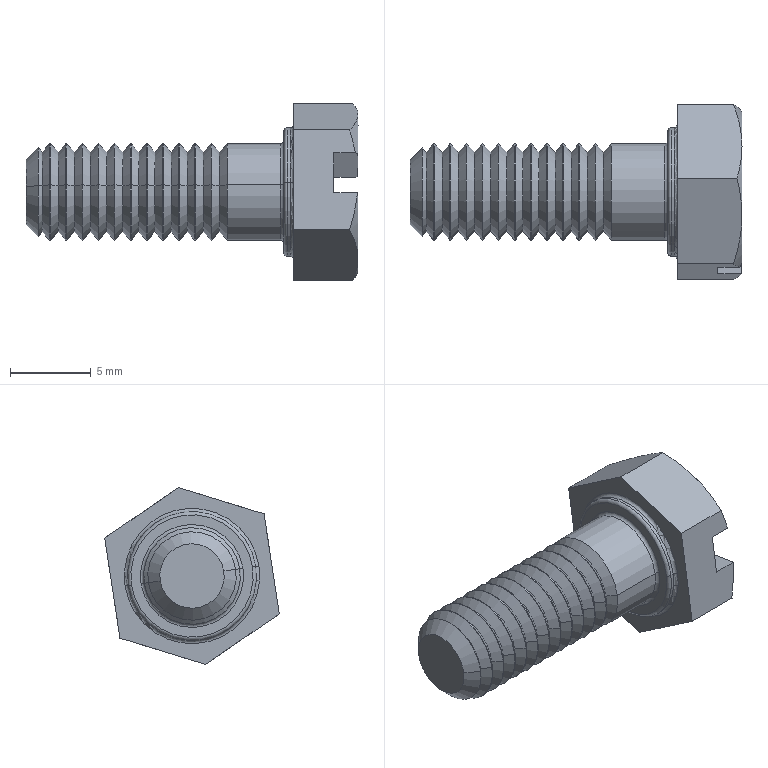Part | SolidWorks | features BaseBody 1 | 1 solid | 106 faces | box 20.6 x 10.831 x 10.98 mm | volume 730.007 mm3 | cone 56 | cylinder 26 | plane 18 | torus 6 | commonest cylinder face diameters 6 x24 8 x2